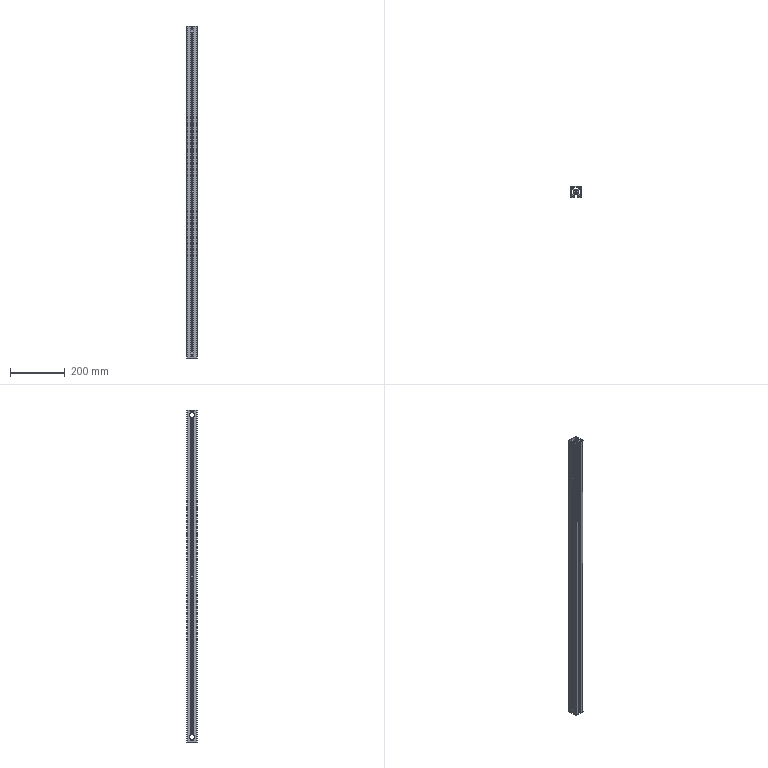Part | SolidWorks | features BaseBody 1, HoleWzd 1, MoveFace 1 | 1 solid | 242 faces | box 40 x 40 x 1210 mm | volume 708024 mm3 | plane 187 | cylinder 55 | commonest cylinder face diameters 6.8 x15 2 x14 19 x12 1 x6 5 x4 9 x4